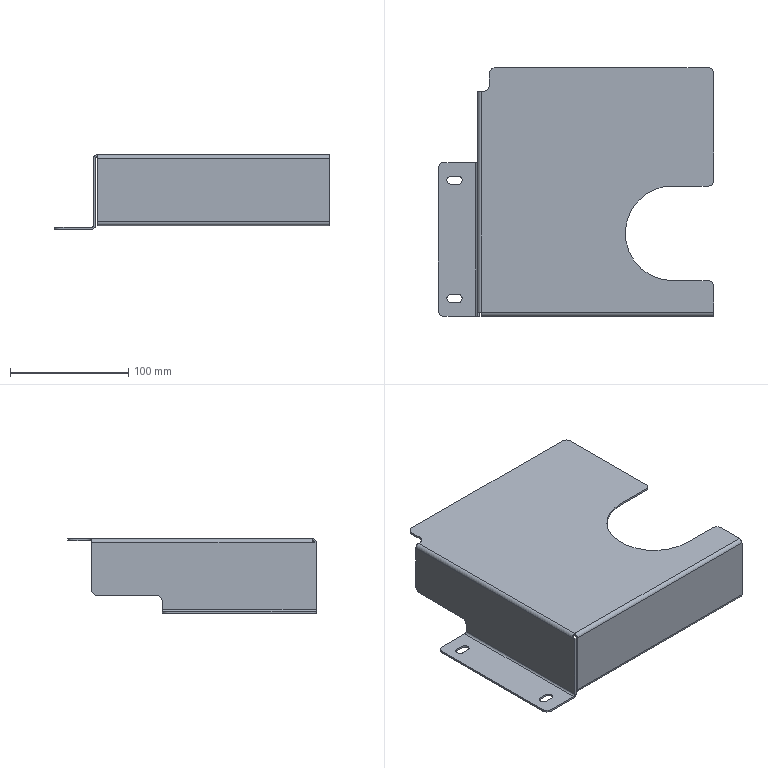Part | STEP file | DCV-000-038 | 1 solid | 76 faces | box 233.4 x 210 x 63 mm | volume 105230 mm3 | plane 42 | cylinder 34 | commonest cylinder face diameters 10 x20 3.2 x4 6.4 x4 7 x4 80 x2